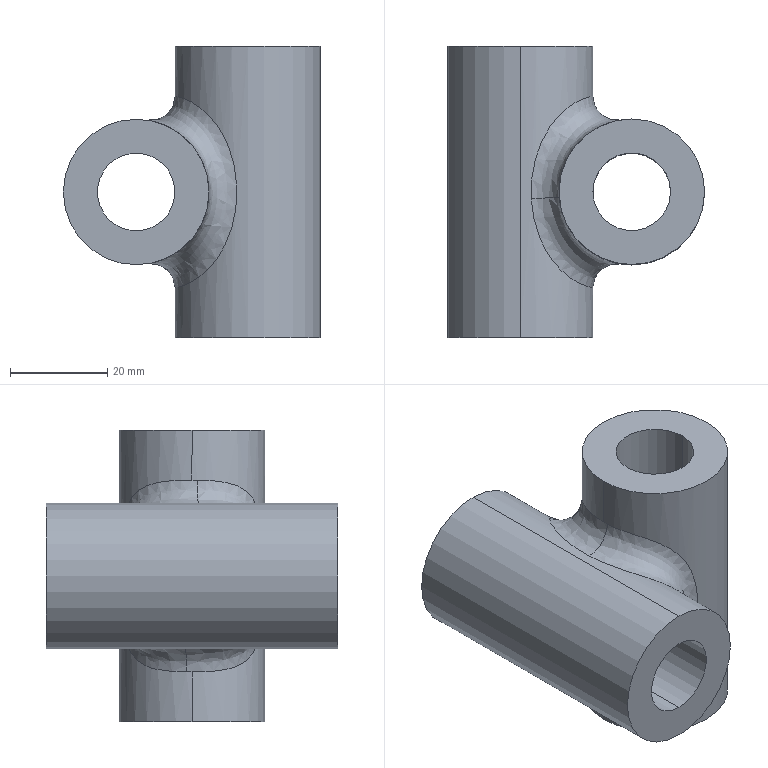Part | SolidWorks | features Extrusion 1, Fillet 1, ICE 1 | 1 solid | 14 faces | box 53 x 60 x 60 mm | volume 59937 mm3 | cylinder 8 | plane 4 | spline 2 | commonest cylinder face diameters 16 x4 30 x4